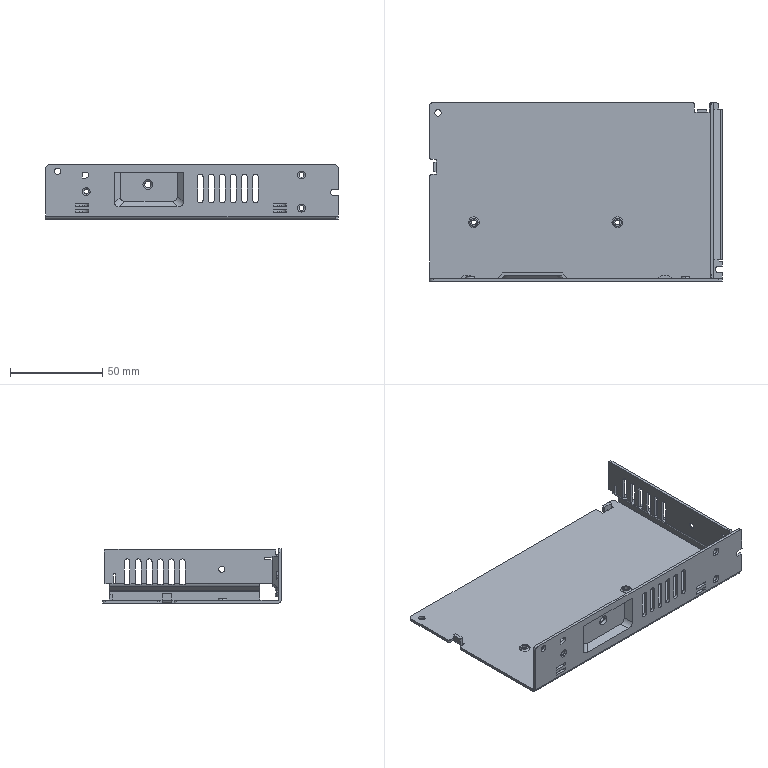Part | STEP file | LRS-150-12_X2_5F00517375-151324 | 1 solid | 288 faces | box 159 x 97 x 29.5 mm | volume 32928 mm3 | plane 153 | cylinder 101 | torus 30 | cone 4 | commonest cylinder face diameters 3 x20 8 x11 2.65 x10 4.27 x10 0.8 x8 3.4 x8